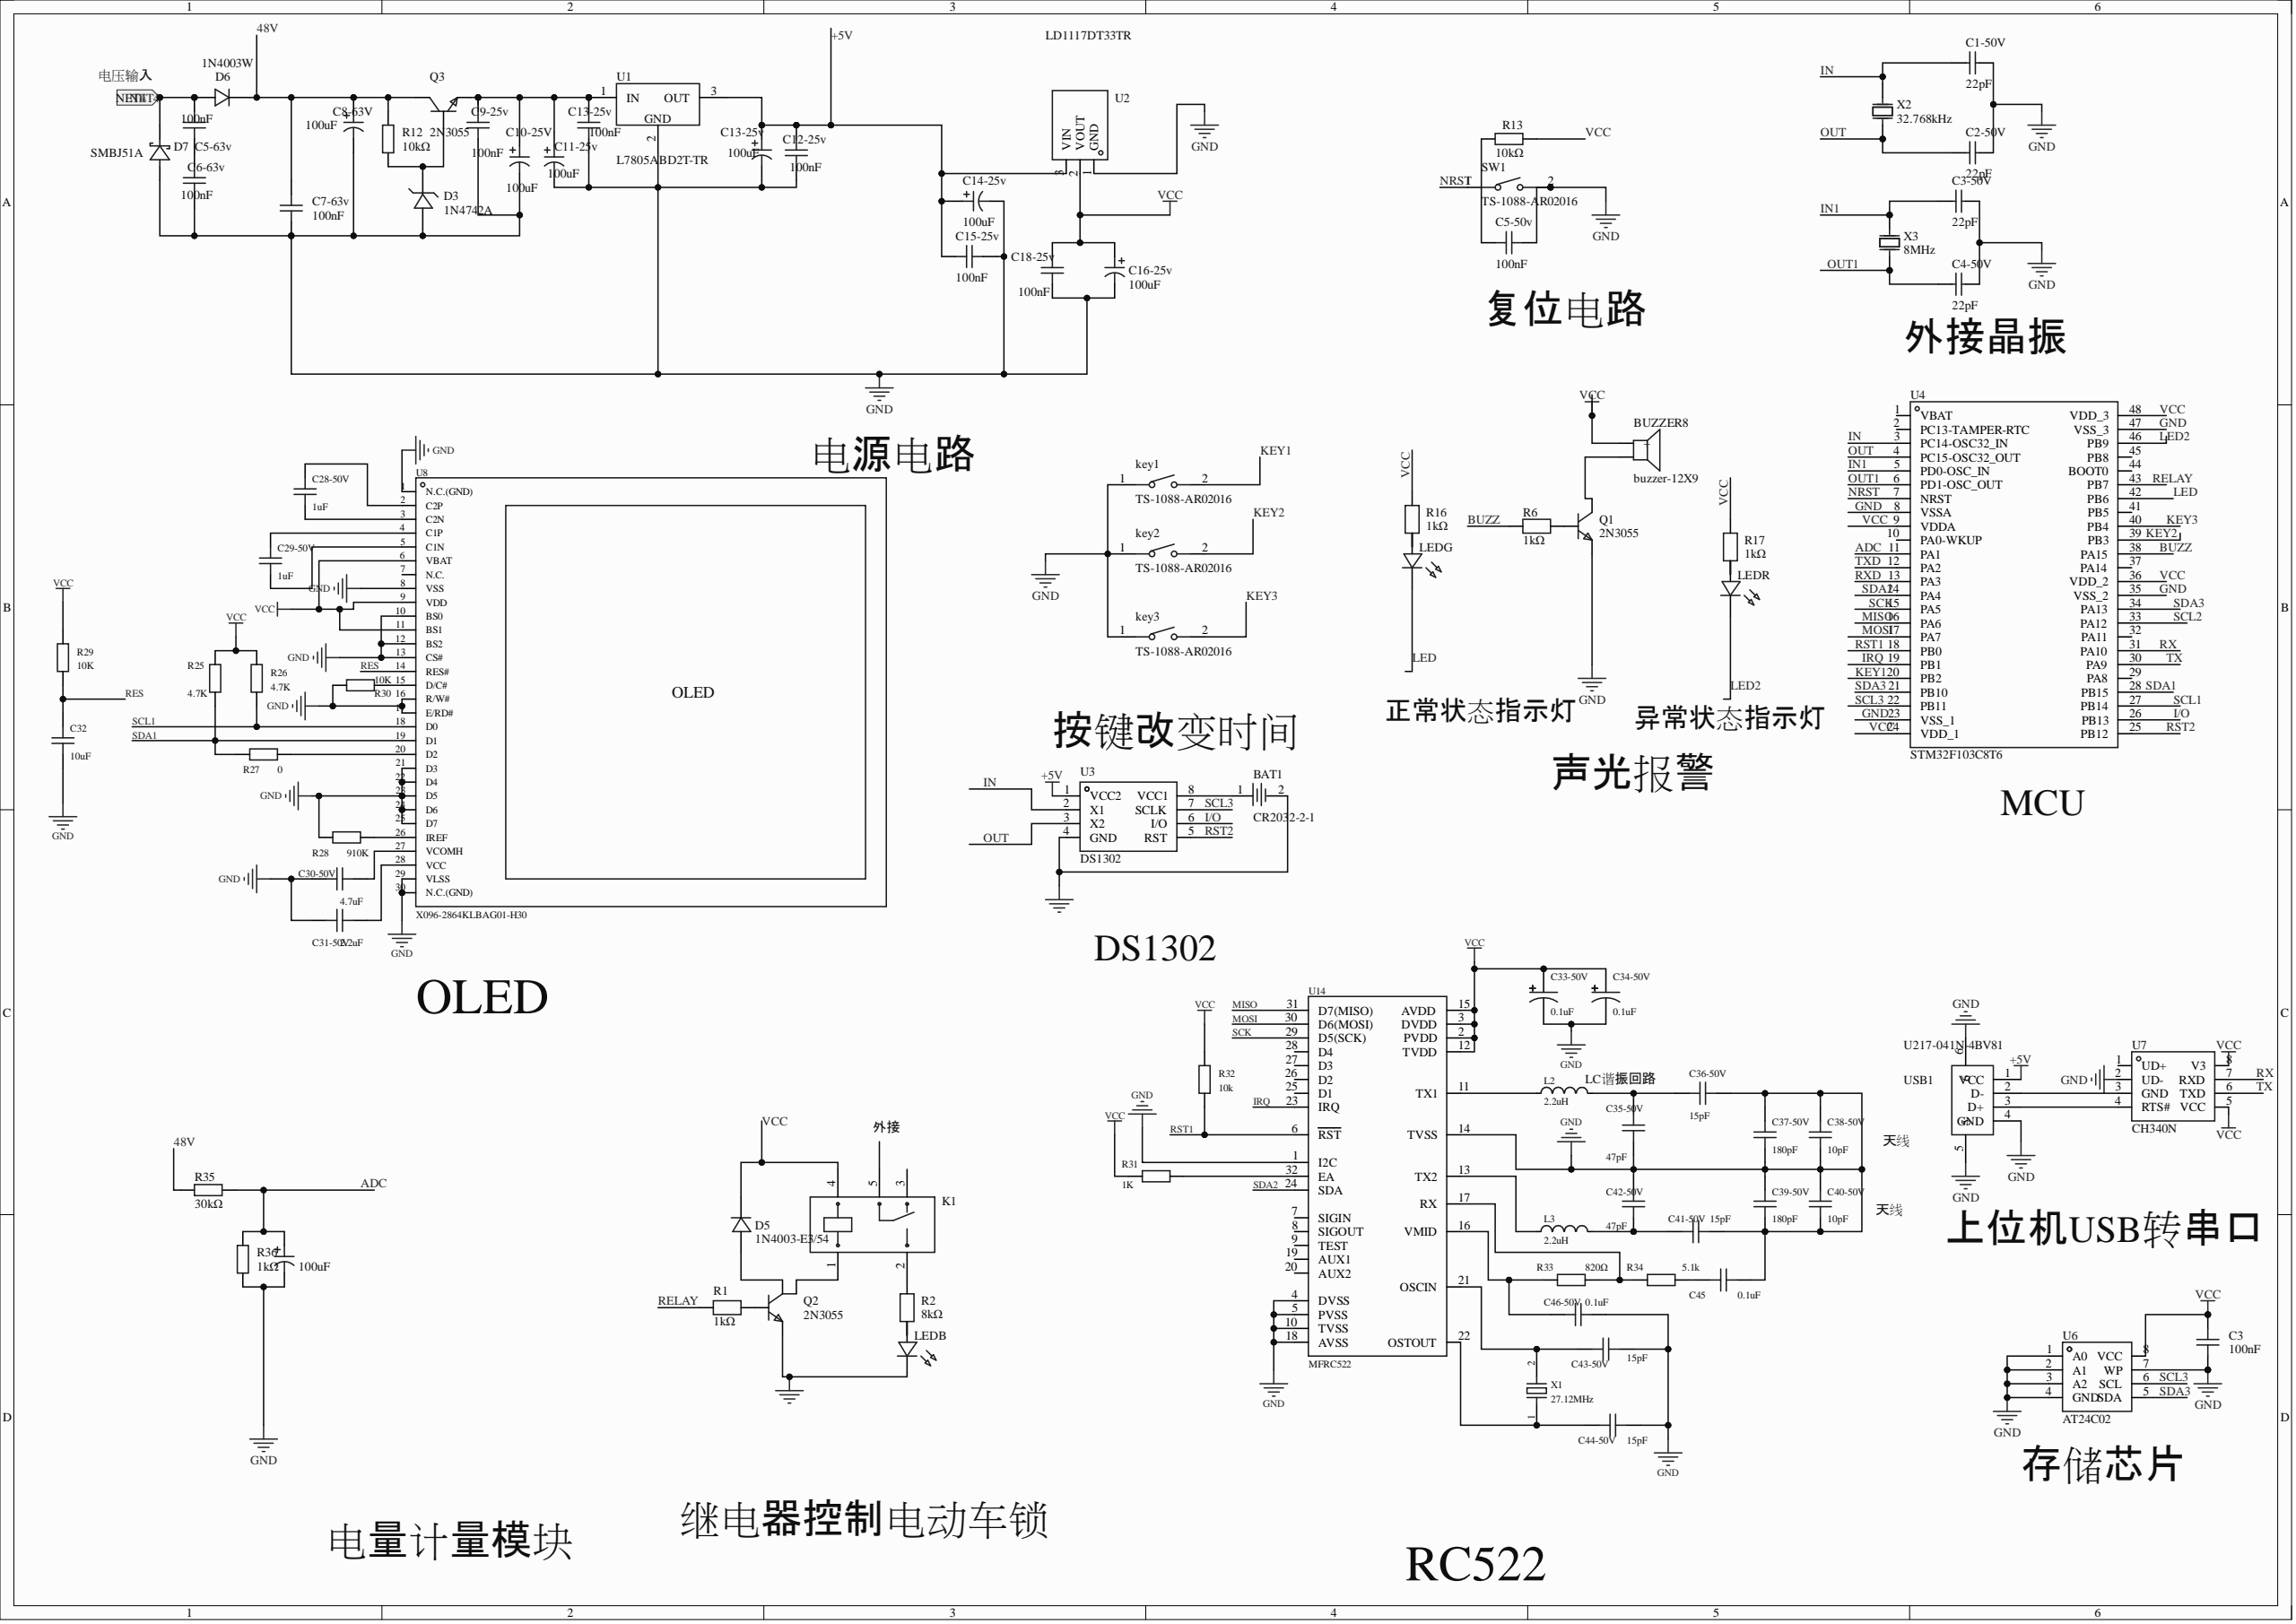Circuit board | Altium Designer | 90 parts | 67 nets
Bill of materials:
Comment,Description,Designator,Footprint,LibRef,Quantity
"CR2032-2-1","","BAT1","BAT-TH_CR2032-2-1","CR2032-2-1","1"
"buzzer-12X9","","BUZZER8","BUZ-TH_BD12.0-P7.60-D0.6-FD","buzzer-12X9","1"
"22pF","容值:22pF;精度:±5%;额定电压:50V;温度系数:C0G;","C1-50V, C2-50V, C3-50V, C4-50V","C0603","CL10C220JB8NNNC","4"
"100nF","","C3, C5-50v, C5-63v, C6-63v","C0603","CAP_0603, CGA0603X7R104K500JT","4"
"100uF","容值:100uF;精度:±20%;额定电压:63V;纹波电流:200mA@120Hz;等效串联电阻(ESR):-;","C5-63v","CAP-SMD_BD10.0-L10.3-W10.3-LS11.0-FD_1","RVT63V100M10X10","1"
"100nF","容值:100nF;精度:±10%;工作电压(AC):275V;防护等级:X2;","C7-63v, C9-25v, C12-25v, C13-25v, C15-25v, C18-25v","CAP-TH_L13.0-W6.0-P10.00-D1.0","MP2104K27C3X6LC","6"
"100uF","容值:100uF;精度:±20%;额定电压:50V;纹波电流:140mA@120Hz;","C8-63V, C10-25V, C11-25v, C13-25v, C14-25v, C16-25v","CAP-SMD_BD6.3-L6.6-W6.6-LS7.3-FD-H7.7","JVJ50V100M6x8","6"
"1uF","","C28-50V, C29-50V","C0603","CAP_0603","2"
"4.7uF","","C30-50V","C0603","CAP_0603","1"
"2.2uF","","C31-50V","C0603","CAP_0603","1"
"10uF","","C32","C0603","CAP_0603","1"
"0.1uF","容值:4.7uF;精度:±20%;额定电压:50V;纹波电流:20mA@120Hz;等效串联电阻(ESR):-;","C33-50V, C34-50V","CAP-SMD_BD5.0-L5.3-W5.3-FD","EMVE500ADA4R7ME55G","2"
"47pF","","C35-50V, C42-50V","C0603","CAP_0603","2"
"15pF","","C36-50V, C41-50V, C43-50V, C44-50V","C0603","CAP_0603","4"
"180pF","","C37-50V, C39-50V","C0603","CAP_0603","2"
"10pF","","C38-50V, C40-50V","C0603","CAP_0603","2"
"0.1uF","","C45, C46-50V","C0603","CAP_0603","2"
"1N4742A","二极管配置:独立式;稳压值(标称值):12V;稳压值(范围):11.4V~12.6V;耗散功率(Pd):1W;","D3","DO-41_BD2.4-L4.7-P8.70-D0.9-RD","1N4742A_C140853","1"
"1N4003-E3/54","二极管配置:-;正向压降(Vf):1.1V@1A;直流反向耐压(Vr):200V;整流电流:1A;","D5","DO-41_BD2.4-L4.7-P8.70-D0.9-RD","1N4003-E3/54","1"
"1N4003W","二极管配置:独立式;正向压降(Vf):1.1V@1A;直流反向耐压(Vr):200V;整流电流:1A;","D6","SOD-123FL_L2.7-W1.8-LS3.8-RD","1N4003W","1"
"SMBJ51A","极性:单向;反向截止电压(Vrwm):51V;钳位电压:82.4V;峰值脉冲电流(Ipp):7.3A@10/1000us;峰值脉冲功率(Ppp):600W@10/1000us;击穿电压:62.7V;","D7","SMB_L4.3-W3.6-LS5.4-R-RD","SMBJ51A_C1973217","1"
"","继电器类型:-;线圈类型:-;线圈电压:-;触点形式:-;触点的额定电流:-;","K1","RELAY-TH_SRD-DCXXV-SL-C","SRD-DC5V-SL-C","1"
"TS-1088-AR02016","电路结构:单刀单掷;按钮形状:圆形按钮;作用力:1.6N;安装方式:立贴;开关长度:4mm;开关宽度:3mm;开关高度:2mm;带支架:不带支架;触点电流:50mA;额定电压:12V;工作寿命:10万次;","key1, key2, key3, SW1","SW-SMD_L3.9-W3.0-P4.45","TS-1088-AR02016","4"
"2.2uH","","L2, L3","L0603","L_0603","2"
"","","LEDB, LEDG, LEDR","LED_TH-3mm","LED_TH-B_3mm","3"
"2N3055","晶体管类型:NPN;集电极电流(Ic):15A;集射极击穿电压(Vceo):60V;耗散功率(Pd):115W;直流电流增益(hFE):5@10A,4V;","Q1, Q2, Q3","TO-3_L39.4-W26.7-P10.92-BL","2N3055_C2848354","3"
"","","R1, R2, R6, R16, R17","RES-TH_BD2.3-L6.5-P10.50-D0.5","插件电阻","5"
"10kΩ","","R12, R13","R0805","0805W8F1002T5E_C17414","2"
"4.7K","","R25, R26","R0603","Res_0603","2"
"0","","R27","R0603","Res_0603","1"
"910K","","R28","R0603","Res_0603","1"
"10K","","R29, R30, R32","R0603","Res_0603","3"
"1K","","R31","R0603","Res_0603","1"
"820Ω","","R33","R0603","Res_0603","1"
"5.1k","","R34","R0603","Res_0603","1"
"30kΩ","","R35","R0603","0603WAF3002T5E","1"
"1kΩ","","R36","R0603","0603WAF1001T5E","1"
"L7805ABD2T-TR","输出类型:固定;工作电压:35V;输出电压:5V;输出电流:1.5A;电源纹波抑制比(PSRR):68dB@(120Hz);输出极性:正极;","U1","TO-263-2_L10.0-W9.2-P5.08-LS15.3-TL-CW","L7805ABD2T-TR","1"
"LD1117DT33TR","输出类型:固定;工作电压:15V;输出电压:3.3V;输出电流:800mA;电源纹波抑制比(PSRR):75dB@(120Hz);输出极性:正极;","U2","TO-252-2_L6.6-W6.1-P4.57-LS9.9-BR-CW","LD1117DT33TR","1"
"DS1302","","U3","DIP-8_L9.7-W6.4-P2.54-LS7.6-BL","DS1302N","1"
"STM32F103C8T6","CPU内核:ARM-M3;CPU最大主频:72MHz;应用领域:-;","U4","LQFP-48_L7.0-W7.0-P0.50-LS9.0-BL","STM32F103C8T6","1"
"MFRC522","","U5","QFN32","MFRC522","1"
"AT24C02","","U6","SOIC-8_L4.9-W3.9-P1.27-LS6.0-BL","AT24C02","1"
"CH340N","应用功能:USB转串口;USB协议版本:USB 2.0;通道数:1;数据速率:2Mbps;","U7","SOP-8_L4.9-W3.9-P1.27-LS6.0-BL","CH340N","1"
"X096-2864KLBAG01-H30","核心芯片:SSD1315;尺寸(inch):0.96;像素分辨率:128x64;","U8","OLED-SMD_X096-2864KLBAG01-H30","X096-2864KLBAG01-H30","1"
"U217-041N-4BV81","连接器类型:Type-A;标准:USB 2.0;公母:公头;触点数量:4;端口数量:1;安装方式:沉板;额定电流 - 电源:1.5A;触头材质:黄铜;触头镀层:金;工作温度范围:-40℃~+85℃;焊接温度(最大值):260℃;","USB1","USB-A-SMD_U217-041N-4BV81","U217-041N-4BV81","1"
"27.12MHz","晶振类型:贴片晶振;频率:27.12MHz;常温频差:±20ppm;负载电容:20pF;频率稳定度:±20ppm;","X1","OSC-SMD_L11.4-W4.5-LS12.5","XJHCCLNANF-27.12MHZ","1"
"32.768kHz","晶振类型:贴片晶振;频率:32.768kHz;常温频差:±20ppm;负载电容:12.5pF;频率稳定度:±30ppm;","X2","CRYSTAL-SMD_L3.2-W1.5-1","XKXGI-SUA-32.768K","1"
"8MHz","晶振类型:贴片晶振;频率:8MHz;常温频差:±10ppm;负载电容:20pF;频率稳定度:±20ppm;","X3","CRYSTAL-SMD_L5.0-W3.2","X50328MSB2GI","1"
Netlist (Protel format):
[
BAT1
BAT-TH_CR2032-2-1
CR2032-2-1



]
[
BUZZER8
BUZ-TH_BD12.0-P7.60-D0.6-FD
buzzer-12X9



]
[
C1-50V
C0603
22pF



]
[
C2-50V
C0603
22pF



]
[
C3
C0603
100nF



]
[
C3-50V
C0603
22pF



]
[
C4-50V
C0603
22pF



]
[
C5-50v
C0603
100nF



]
[
C5-63v
CAP-SMD_BD10.0-L10.3-W10.3-LS11.0-FD_1
100uF



]
[
C5-63v
C0603
100nF



]
[
C6-63v
C0603
100nF



]
[
C7-63v
CAP-TH_L13.0-W6.0-P10.00-D1.0
100nF



]
[
C8-63V
CAP-SMD_BD6.3-L6.6-W6.6-LS7.3-FD-H7.7
100uF



]
[
C9-25v
CAP-TH_L13.0-W6.0-P10.00-D1.0
100nF



]
[
C10-25V
CAP-SMD_BD6.3-L6.6-W6.6-LS7.3-FD-H7.7
100uF



]
[
C11-25v
CAP-SMD_BD6.3-L6.6-W6.6-LS7.3-FD-H7.7
100uF



]
[
C12-25v
CAP-TH_L13.0-W6.0-P10.00-D1.0
100nF



]
[
C13-25v
CAP-SMD_BD6.3-L6.6-W6.6-LS7.3-FD-H7.7
100uF



]
[
C13-25v
CAP-TH_L13.0-W6.0-P10.00-D1.0
100nF



]
[
C14-25v
CAP-SMD_BD6.3-L6.6-W6.6-LS7.3-FD-H7.7
100uF



]
[
C15-25v
CAP-TH_L13.0-W6.0-P10.00-D1.0
100nF



]
[
C16-25v
CAP-SMD_BD6.3-L6.6-W6.6-LS7.3-FD-H7.7
100uF



]
[
C18-25v
CAP-TH_L13.0-W6.0-P10.00-D1.0
100nF



]
[
C28-50V
C0603
1uF



]
[
C29-50V
C0603
1uF



]
[
C30-50V
C0603
4.7uF



]
[
C31-50V
C0603
2.2uF



]
[
C32
C0603
10uF



]
[
C33-50V
CAP-SMD_BD5.0-L5.3-W5.3-FD
0.1uF



]
[
C34-50V
CAP-SMD_BD5.0-L5.3-W5.3-FD
0.1uF



]
[
C35-50V
C0603
47pF



]
[
C36-50V
C0603
15pF



]
[
C37-50V
C0603
180pF



]
[
C38-50V
C0603
10pF



]
[
C39-50V
C0603
180pF



]
[
C40-50V
C0603
10pF



]
[
C41-50V
C0603
15pF



]
[
C42-50V
C0603
47pF



]
[
C43-50V
C0603
15pF



]
[
C44-50V
C0603
15pF



]
[
C45
C0603
0.1uF



]
[
C46-50V
C0603
0.1uF



]
[
D3
DO-41_BD2.4-L4.7-P8.70-D0.9-RD
1N4742A



]
[
D5
DO-41_BD2.4-L4.7-P8.70-D0.9-RD
1N4003-E3/54



]
[
D6
SOD-123FL_L2.7-W1.8-LS3.8-RD
1N4003W



]
[
D7
SMB_L4.3-W3.6-LS5.4-R-RD
SMBJ51A



]
[
K1
RELAY-TH_SRD-DCXXV-SL-C




]
[
key1
SW-SMD_L3.9-W3.0-P4.45
TS-1088-AR02016



]
[
key2
SW-SMD_L3.9-W3.0-P4.45
TS-1088-AR02016



]
[
key3
SW-SMD_L3.9-W3.0-P4.45
TS-1088-AR02016



]
[
L2
L0603
2.2uH



]
[
L3
L0603
2.2uH



]
[
LEDB
LED_TH-3mm




]
[
LEDG
LED_TH-3mm




]
[
LEDR
LED_TH-3mm




]
[
Q1
TO-3_L39.4-W26.7-P10.92-BL
2N3055



]
[
Q2
TO-3_L39.4-W26.7-P10.92-BL
2N3055



]
[
Q3
TO-3_L39.4-W26.7-P10.92-BL
2N3055



]
[
R1
RES-TH_BD2.3-L6.5-P10.50-D0.5




]
[
R2
RES-TH_BD2.3-L6.5-P10.50-D0.5




]
[
R6
RES-TH_BD2.3-L6.5-P10.50-D0.5




]
[
R12
R0805
10kΩ



]
[
R13
R0805
10kΩ



]
[
R16
RES-TH_BD2.3-L6.5-P10.50-D0.5




]
[
R17
RES-TH_BD2.3-L6.5-P10.50-D0.5




]
[
R25
R0603
4.7K



]
[
R26
R0603
4.7K



]
[
R27
R0603
0



]
[
R28
R0603
910K



]
[
R29
R0603
10K



]
[
R30
R0603
10K



]
[
R31
R0603
1K



]
[
R32
R0603
10k



]
[
R33
R0603
820Ω



]
[
R34
R0603
5.1k



]
[
R35
R0603
30kΩ



]
[
R36
R0603
1kΩ



]
[
SW1
SW-SMD_L3.9-W3.0-P4.45
TS-1088-AR02016



]
[
U1
TO-263-2_L10.0-W9.2-P5.08-LS15.3-TL-CW
L7805ABD2T-TR



]
[
U2
TO-252-2_L6.6-W6.1-P4.57-LS9.9-BR-CW
LD1117DT33TR



]
[
U3
DIP-8_L9.7-W6.4-P2.54-LS7.6-BL
DS1302



]
[
U4
LQFP-48_L7.0-W7.0-P0.50-LS9.0-BL
STM32F103C8T6



]
[
U5
QFN32
MFRC522



]
[
U6
SOIC-8_L4.9-W3.9-P1.27-LS6.0-BL
AT24C02



]
[
U7
SOP-8_L4.9-W3.9-P1.27-LS6.0-BL
CH340N



]
[
U8
OLED-SMD_X096-2864KLBAG01-H30
X096-2864KLBAG01-H30



]
[
USB1
USB-A-SMD_U217-041N-4BV81
U217-041N-4BV81



]
[
X1
OSC-SMD_L11.4-W4.5-LS12.5
27.12MHz



]
[
X2
CRYSTAL-SMD_L3.2-W1.5-1
32.768kHz



]
[
X3
CRYSTAL-SMD_L5.0-W3.2
8MHz



]
(
TX
U4-30
U7-6
)
(
SDA3
U4-21
U4-34
U6-5
)
(
SDA2
U4-14
U5-24
)
(
SDA1
R25-1
R27-1
U4-28
U8-19
)
(
SCL3
U3-7
U4-22
U6-6
)
(
SCL1
R26-1
U4-27
U8-18
)
(
SCK
U4-15
U5-29
)
(
RX
U4-31
U7-7
)
(
RST2
U3-5
U4-25
)
(
RST1
R32-1
U4-18
U5-6
)
(
RES
C32-2
R29-1
U8-14
)
(
RELAY
R1-1
U4-43
)
(
OUT1
C4-50V-1
U4-6
X3-1
)
(
OUT
C2-50V-1
U3-3
U4-4
X2-1
)
(
NRST
SW1-1
U4-7
)
(
NetU7_4
U7-4
USB1-3
)
(
NetU7_3
U7-3
USB1-2
)
(
NetR33_2
R33-2
R34-1
U5-17
)
(
NetR31_2
R31-2
U5-32
)
(
NetR30_1
R30-1
U8-15
)
(
NetR28_2
R28-2
U8-26
)
(
NetR27_2
R27-2
U8-20
)
(
NetQ2_1
Q2-1
R1-2
)
(
NetQ1_1
Q1-1
R6-2
)
(
NetLEDR_1
LEDR-1
R17-1
)
(
NetLEDG_1
LEDG-1
R16-1
)
(
NetLEDB_1
LEDB-1
R2-1
)
(
NetL3_1
L3-1
U5-13
)
(
NetL2_1
L2-1
U5-11
)
(
NetK1_2
K1-2
R2-2
)
(
NetK1_1
K1-1
Q2-4
)
(
NetD5_2
D5-2
Q2-3
)
(
NetD3_1
D3-1
Q3-1
R12-1
)
(
NetC46-50V_1
C46-50V-1
R33-1
U5-16
)
(
NetC45_2
C45-2
R34-2
)
(
NetC44-50V_2
C44-50V-2
U5-22
X1-1
)
(
NetC43-50V_2
C43-50V-2
U5-21
X1-2
)
(
NetC41-50V_1
C41-50V-1
C42-50V-1
L3-2
)
(
NetC35-50V_2
C35-50V-2
C36-50V-1
L2-2
)
(
NetC31-50V_2
C31-50V-2
U8-28
)
(
NetC30-50V_2
C30-50V-2
U8-27
)
(
NetC29-50V_2
C29-50V-2
U8-4
)
(
NetC29-50V_1
C29-50V-1
U8-5
)
(
NetC28-50V_2
C28-50V-2
U8-2
)
(
NetC28-50V_1
C28-50V-1
U8-3
)
(
NetC9-25v_1
C9-25v-1
C10-25V-1
C11-25v-1
C13-25v-1
Q3-2
U1-1
)
(
NetC5-63v_1
C5-63v-1
C6-63v-2
)
(
NetC5-50v_1
C5-50v-1
R13-2
)
(
NetBUZZER8_2
BUZZER8-2
Q1-3
)
(
NetBAT1_1
BAT1-1
U3-8
)
(
NET4
C5-63v-2
D6-2
D7-2
)
(
MOSI
U4-17
U5-30
)
(
MISO
U4-16
U5-31
)
(
LED2
LEDR-2
U4-46
)
(
LED
LEDG-2
U4-42
)
(
KEY3
key3-2
U4-40
)
(
KEY2
key2-2
U4-39
)
(
KEY1
key1-2
U4-20
)
(
IRQ
U4-19
U5-23
)
(
IN1
C3-50V-1
U4-5
X3-2
)
(
IN
C1-50V-1
U3-2
U4-3
X2-2
)
(
I/O
U3-6
U4-26
)
(
GND
BAT1-2
BUZZER8-1
C1-50V-2
C2-50V-2
C3-1
C3-2
C3-50V-2
C4-50V-2
C5-50v-2
C5-63v-2
C6-63v-1
C7-63v-2
C8-63V-2
C9-25v-2
C10-25V-2
C11-25v-2
C12-25v-2
C13-25v-2
C13-25v-2
C14-25v-2
C15-25v-1
C16-25v-1
C16-25v-2
C18-25v-1
C18-25v-2
C30-50V-1
C31-50V-1
C32-1
C33-50V-1
C33-50V-2
C34-50V-1
C34-50V-2
C35-50V-1
C36-50V-2
C37-50V-1
C37-50V-2
C38-50V-1
C38-50V-2
C39-50V-1
C39-50V-2
C40-50V-1
C40-50V-2
C41-50V-2
C42-50V-2
C43-50V-1
C44-50V-1
C45-1
C46-50V-2
D3-2
D5-1
D7-1
K1-4
key1-1
key2-1
key3-1
LEDB-2
Q1-2
Q2-2
R13-1
R16-2
R17-2
R25-2
R26-2
R28-1
R29-2
R30-2
R31-1
R32-2
R36-1
SW1-2
U1-2
U2-1
U2-2
U3-4
U4-8
U4-9
U4-23
U4-24
U4-35
U4-36
U4-47
U4-48
U5-1
U5-2
U5-3
U5-4
U5-5
U5-10
U5-12
U5-14
U5-15
U5-18
U6-1
U6-2
U6-3
U6-4
U6-7
U6-8
U7-2
U7-5
U7-8
U8-1
U8-6
U8-8
U8-9
U8-10
U8-11
U8-12
U8-13
U8-16
U8-17
U8-21
U8-22
U8-23
U8-24
U8-25
U8-29
U8-30
USB1-4
USB1-5
USB1-6
)
(
BUZZ
R6-1
U4-38
)
(
ADC
C5-63v-1
R35-2
R36-2
U4-11
)
(
+5V
C12-25v-1
C13-25v-1
C14-25v-1
C15-25v-2
U1-3
U2-3
U3-1
USB1-1
)
(
48V
C7-63v-1
C8-63V-1
D6-1
Q3-3
R12-2
R35-1
)